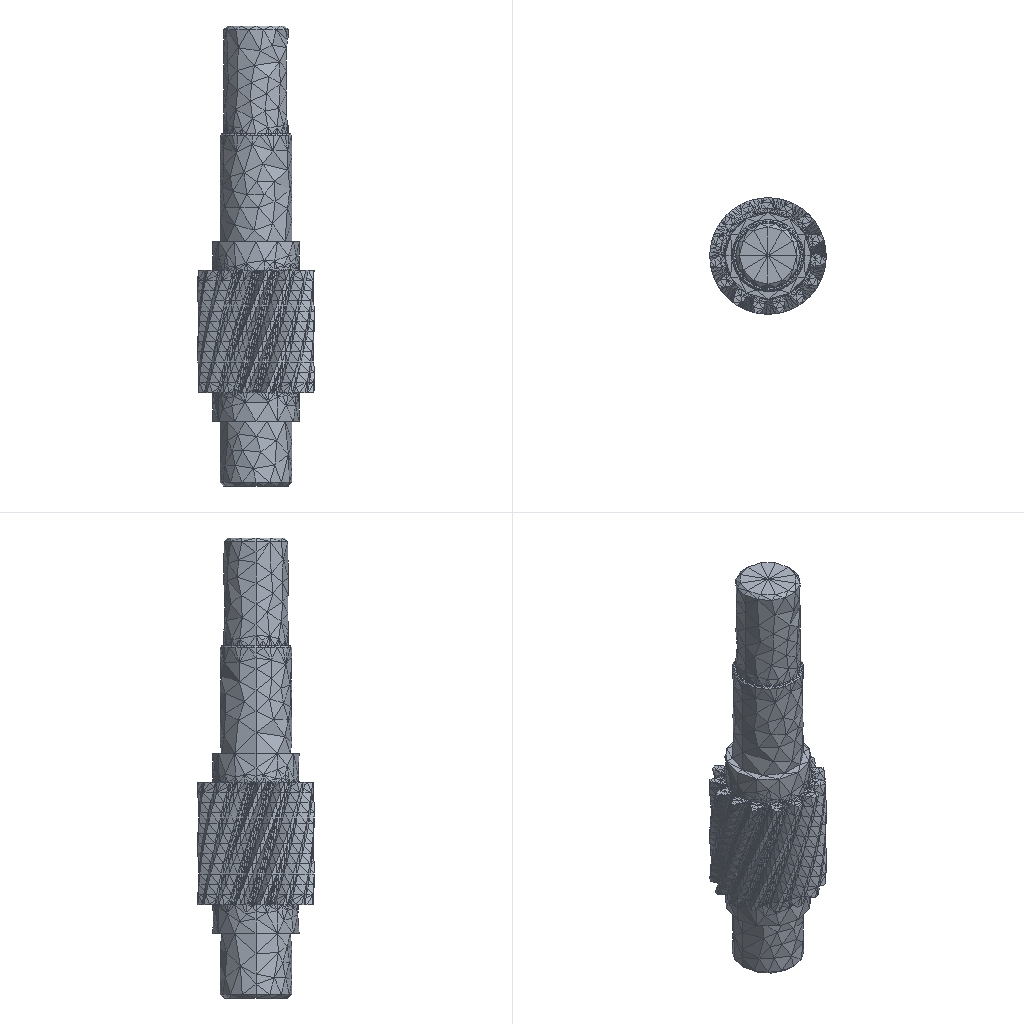Simulation study | ansys workbench
Ansys APDL input file, long lists of numbers shortened:
/batch
/config,noeldb,1     ! force off writing results to database
*get,_wallstrt,active,,time,wall
! ANSYS input file written by Workbench version 2022 R1
/assign,rstp,file,rst              ! Force Eigen analysis to write to file.rst because WB expects it
/solu
antype,,restart,,,perturbation
*DIM,_wb_ProjectScratch_dir_Modal,string,248
_wb_ProjectScratch_dir_Modal(1)= 'C:\Users\Administrator\AppData\Local\Temp\WB_Administrator_4372_2\_ProjectScratch\ScrEDF1\'
*DIM,_wb_SolverFiles_dir_Modal,string,248
_wb_SolverFiles_dir_Modal(1)= 'C:\Users\Administrator\AppData\Local\Temp\WB_Administrator_4372_2\wbnew_files\dp0\SYS-1\MECH\'
*DIM,_wb_userfiles_dir_Modal,string,248
_wb_userfiles_dir_Modal(1)= 'C:\Users\Administrator\AppData\Local\Temp\WB_Administrator_4372_2\wbnew_files\user_files\'
/title,wbnew--__ (C5)
! ****** Begin Custom Load Command Snippet ******
/COM, ACT Extensions:
/COM,     LSDYNA, 2021.1
/COM,
! ****** End   Custom Load Command Snippet ******
perturb,modal,,CURRENT,DZEROKEEP          ! pre-stress modal analysis, only keep zero bcs in case future MSUP
solve, elform                                       ! Generate matrices needed for perturbation analysis
_thickRatio=  1     ! Ratio of thick parts in the model
modopt,lanb,6
outres,erase
outres,all,none
outres,nsol,all
outres,etmp,all
mxpand                    ! default expand in case of complex solution
dmpopt,esav,no
dmpopt,emat,no
dmpopt,full,no
! *********** WB SOLVE COMMAND ***********
! check interactive state
*get,ANSINTER_,active,,int
*if,ANSINTER_,ne,0,then
/eof
*endif
solve
/com *************** Write FE CONNECTORS *********
CEWRITE,file,ce,,INTE
*get,_nmodalsolproc,active,0,numcpu
fini
/nopr
*get,_numnode,node,0,count
*get,_numelem,elem,0,count
*get, _MAXELEMNUM, elem, 0, NUM, MAX
*get, _MAXNODENUM, node, 0, NUM, MAX,,,INTERNAL
*get, _MAXELEMTYPE, etyp, 0, NUM, MAX
*get, _MAXREALCONST, real, 0, NUM, MAX
/gopr
*get,_wallasol,active,,time,wall
/post1
/nopr
*dim,_direction,CHAR,6,1
_direction(1) = 'X'
_direction(2) = 'Y'
_direction(3) = 'Z'
_direction(4) = 'ROTX'
_direction(5) = 'ROTY'
_direction(6) = 'ROTZ'
*get,_lastLS,active,0,set,LSTP
*get,_beginset,active,0,set,nset,first,_lastLS
*get,_endset,active,0,set,nset,last,_lastLS
_nummodes = 0
*if,_endset,gt,0,then
_nummodes = _endset - _beginset + 1
*endif
*do,i_mode,1,_nummodes
   *do,j_component,1,6
			*get,PFACT_%i_mode%_%j_component%,MODE,%i_mode%,PFACT,,DIREC,_direction(%j_component%)
   *enddo
*enddo
*dim,_tmdirection,CHAR,6,1
_tmdirection(1) = 'X'
_tmdirection(2) = 'Y'
_tmdirection(3) = 'Z'
_tmdirection(4) = 'X'
_tmdirection(5) = 'Y'
_tmdirection(6) = 'Z'
*do,j_component,1,6
    *if,j_component,gt,3,then
        *get,TOTALMASS_%j_component%,ELEM,0,IOR,_tmdirection(%j_component%)
    *else
        *get,TOTALMASS_%j_component%,ELEM,0,MTOT,_tmdirection(%j_component%)
    *endif
*enddo
/gopr
xmlo,ENCODING,ISO-8859-1
xmlo,parm
/xml,parm,xml
fini
/gopr
*get,_walldone,active,,time,wall
_preptime=(_wallbsol-_wallstrt)*3600
_solvtime=(_wallasol-_wallbsol)*3600
_posttime=(_walldone-_wallasol)*3600
_totaltim=(_walldone-_wallstrt)*3600
*get,_dlbratio,active,0,solu,dlbr
*get,_combtime,active,0,solu,comb
*get,_ssmode,active,0,solu,ssmm
*get,_ndofs,active,0,solu,ndof
/fclean				!clean distributed files
/com,--- Total number of nodes = %_numnode%
/com,--- Total number of elements = %_numelem%
/com,--- Element load balance ratio = %_dlbratio%
/com,--- Time to combine distributed files = %_combtime%
/com,--- Sparse memory mode = %_ssmode%
/com,--- Number of DOF = %_ndofs%
/wb,file,end               ! done with WB generated input